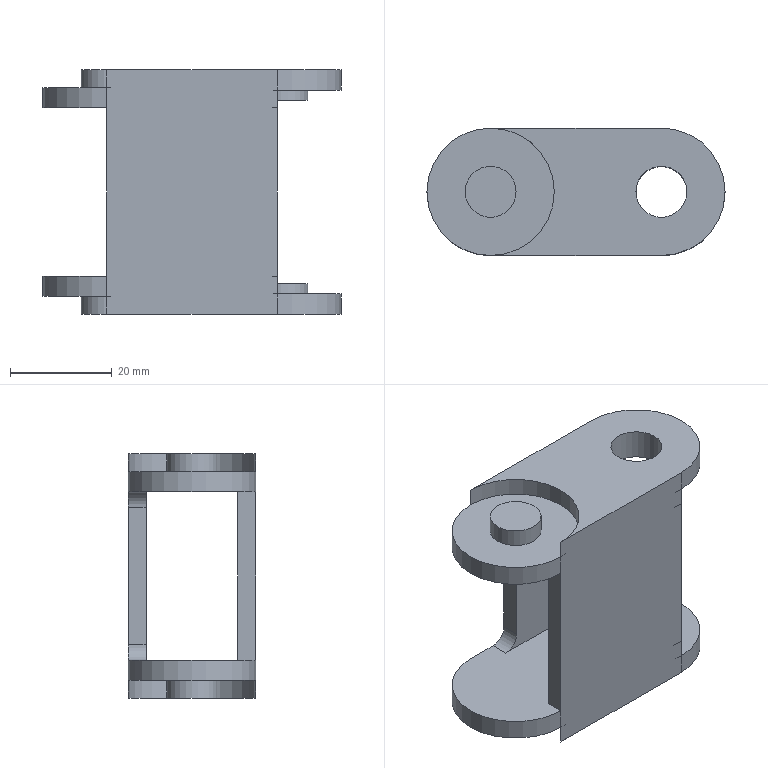Part | STEP file | 1 solid | 42 faces | box 58.5 x 25 x 48 mm | volume 18741 mm3 | plane 24 | cylinder 18 | commonest cylinder face diameters 25 x8 6 x4 10 x4 12 x2